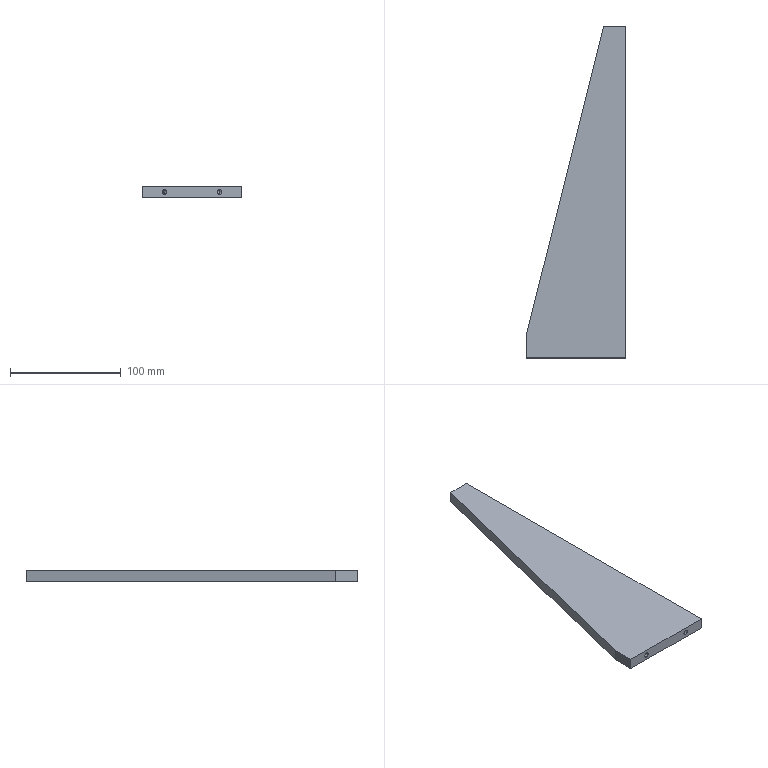Part | SolidWorks | features HoleWzd 2, Extrusion 1, ICE 1 | 1 solid | 23 faces | box 90 x 300 x 10 mm | volume 171179 mm3 | cylinder 8 | cone 8 | plane 7 | commonest cylinder face diameters 4.2 x8
STEP:
#1=CARTESIAN_POINT('',(30.6,110.,7.1));
#2=VERTEX_POINT('',#1);
#3=CARTESIAN_POINT('',(30.6,110.,2.9));
#4=VERTEX_POINT('',#3);
#5=CARTESIAN_POINT('',(30.6,110.,5.));
#6=DIRECTION('',(1.,0.,0.));
#7=DIRECTION('',(0.,0.,-1.));
#8=AXIS2_PLACEMENT_3D('',#5,#6,#7);
#9=CIRCLE('',#8,2.1);
#10=EDGE_CURVE('',#2,#4,#9,.T.);
#11=ORIENTED_EDGE('',*,*,#10,.F.);
#12=CARTESIAN_POINT('',(45.,110.,7.1));
#13=VERTEX_POINT('',#12);
#14=CARTESIAN_POINT('',(45.,110.,7.1));
#15=DIRECTION('',(1.,0.,0.));
#16=VECTOR('',#15,1000.);
#17=LINE('',#14,#16);
#18=EDGE_CURVE('',#2,#13,#17,.T.);
#19=ORIENTED_EDGE('',*,*,#18,.T.);
#20=CARTESIAN_POINT('',(45.,110.,2.9));
#21=VERTEX_POINT('',#20);
#22=CARTESIAN_POINT('',(45.,110.,5.));
#23=DIRECTION('',(1.,0.,0.));
#24=DIRECTION('',(0.,0.,-1.));
#25=AXIS2_PLACEMENT_3D('',#22,#23,#24);
#26=CIRCLE('',#25,2.1);
#27=EDGE_CURVE('',#13,#21,#26,.T.);
#28=ORIENTED_EDGE('',*,*,#27,.T.);
#29=CARTESIAN_POINT('',(45.,110.,2.9));
#30=DIRECTION('',(1.,0.,0.));
#31=VECTOR('',#30,1000.);
#32=LINE('',#29,#31);
#33=EDGE_CURVE('',#4,#21,#32,.T.);
#34=ORIENTED_EDGE('',*,*,#33,.F.);
#35=EDGE_LOOP('',(#11,#19,#28,#34));
#36=FACE_OUTER_BOUND('',#35,.T.);
#37=CARTESIAN_POINT('',(45.,110.,5.));
#38=DIRECTION('',(1.,0.,0.));
#39=DIRECTION('',(0.,0.,-1.));
#40=AXIS2_PLACEMENT_3D('',#37,#38,#39);
#41=CYLINDRICAL_SURFACE('',#40,2.1);
#42=ADVANCED_FACE('',(#36),#41,.F.);
#43=CARTESIAN_POINT('',(29.338,110.,5.));
#44=VERTEX_POINT('',#43);
#45=CARTESIAN_POINT('',(30.6,110.,2.9));
#46=DIRECTION('',(0.515,0.,-0.8572));
#47=VECTOR('',#46,1000.);
#48=LINE('',#45,#47);
#49=EDGE_CURVE('',#44,#4,#48,.T.);
#50=ORIENTED_EDGE('',*,*,#49,.F.);
#51=CARTESIAN_POINT('',(30.6,110.,7.1));
#52=DIRECTION('',(0.515,0.,0.8572));
#53=VECTOR('',#52,1000.);
#54=LINE('',#51,#53);
#55=EDGE_CURVE('',#44,#2,#54,.T.);
#56=ORIENTED_EDGE('',*,*,#55,.T.);
#57=ORIENTED_EDGE('',*,*,#10,.T.);
#58=EDGE_LOOP('',(#50,#56,#57));
#59=FACE_OUTER_BOUND('',#58,.T.);
#60=CARTESIAN_POINT('',(30.6,110.,5.));
#61=DIRECTION('',(1.,0.,0.));
#62=DIRECTION('',(0.,0.,-1.));
#63=AXIS2_PLACEMENT_3D('',#60,#61,#62);
#64=CONICAL_SURFACE('',#63,2.1,1.03);
#65=ADVANCED_FACE('',(#59),#64,.F.);
#66=CARTESIAN_POINT('',(30.6,10.,7.1));
#67=VERTEX_POINT('',#66);
#68=CARTESIAN_POINT('',(30.6,10.,2.9));
#69=VERTEX_POINT('',#68);
#70=CARTESIAN_POINT('',(30.6,10.,5.));
#71=DIRECTION('',(1.,0.,0.));
#72=DIRECTION('',(0.,0.,-1.));
#73=AXIS2_PLACEMENT_3D('',#70,#71,#72);
#74=CIRCLE('',#73,2.1);
#75=EDGE_CURVE('',#67,#69,#74,.T.);
#76=ORIENTED_EDGE('',*,*,#75,.F.);
#77=CARTESIAN_POINT('',(45.,10.,7.1));
#78=VERTEX_POINT('',#77);
#79=CARTESIAN_POINT('',(45.,10.,7.1));
#80=DIRECTION('',(1.,0.,0.));
#81=VECTOR('',#80,1000.);
#82=LINE('',#79,#81);
#83=EDGE_CURVE('',#67,#78,#82,.T.);
#84=ORIENTED_EDGE('',*,*,#83,.T.);
#85=CARTESIAN_POINT('',(45.,10.,2.9));
#86=VERTEX_POINT('',#85);
#87=CARTESIAN_POINT('',(45.,10.,5.));
#88=DIRECTION('',(1.,0.,0.));
#89=DIRECTION('',(0.,0.,-1.));
#90=AXIS2_PLACEMENT_3D('',#87,#88,#89);
#91=CIRCLE('',#90,2.1);
#92=EDGE_CURVE('',#78,#86,#91,.T.);
#93=ORIENTED_EDGE('',*,*,#92,.T.);
#94=CARTESIAN_POINT('',(45.,10.,2.9));
#95=DIRECTION('',(1.,0.,0.));
#96=VECTOR('',#95,1000.);
#97=LINE('',#94,#96);
#98=EDGE_CURVE('',#69,#86,#97,.T.);
#99=ORIENTED_EDGE('',*,*,#98,.F.);
#100=EDGE_LOOP('',(#76,#84,#93,#99));
#101=FACE_OUTER_BOUND('',#100,.T.);
#102=CARTESIAN_POINT('',(45.,10.,5.));
#103=DIRECTION('',(1.,0.,0.));
#104=DIRECTION('',(0.,0.,-1.));
#105=AXIS2_PLACEMENT_3D('',#102,#103,#104);
#106=CYLINDRICAL_SURFACE('',#105,2.1);
#107=ADVANCED_FACE('',(#101),#106,.F.);
#108=CARTESIAN_POINT('',(29.338,10.,5.));
#109=VERTEX_POINT('',#108);
#110=CARTESIAN_POINT('',(30.6,10.,2.9));
#111=DIRECTION('',(0.515,0.,-0.8572));
#112=VECTOR('',#111,1000.);
#113=LINE('',#110,#112);
#114=EDGE_CURVE('',#109,#69,#113,.T.);
#115=ORIENTED_EDGE('',*,*,#114,.F.);
#116=CARTESIAN_POINT('',(30.6,10.,7.1));
#117=DIRECTION('',(0.515,0.,0.8572));
#118=VECTOR('',#117,1000.);
#119=LINE('',#116,#118);
#120=EDGE_CURVE('',#109,#67,#119,.T.);
#121=ORIENTED_EDGE('',*,*,#120,.T.);
#122=ORIENTED_EDGE('',*,*,#75,.T.);
#123=EDGE_LOOP('',(#115,#121,#122));
#124=FACE_OUTER_BOUND('',#123,.T.);
#125=CARTESIAN_POINT('',(30.6,10.,5.));
#126=DIRECTION('',(1.,0.,0.));
#127=DIRECTION('',(0.,0.,-1.));
#128=AXIS2_PLACEMENT_3D('',#125,#126,#127);
#129=CONICAL_SURFACE('',#128,2.1,1.03);
#130=ADVANCED_FACE('',(#124),#129,.F.);
#131=CARTESIAN_POINT('',(25.,-135.6,7.1));
#132=VERTEX_POINT('',#131);
#133=CARTESIAN_POINT('',(25.,-135.6,2.9));
#134=VERTEX_POINT('',#133);
#135=CARTESIAN_POINT('',(25.,-135.6,5.));
#136=DIRECTION('',(0.,-1.,0.));
#137=DIRECTION('',(0.,0.,-1.));
#138=AXIS2_PLACEMENT_3D('',#135,#136,#137);
#139=CIRCLE('',#138,2.1);
#140=EDGE_CURVE('',#132,#134,#139,.T.);
#141=ORIENTED_EDGE('',*,*,#140,.F.);
#142=CARTESIAN_POINT('',(25.,-150.,7.1));
#143=VERTEX_POINT('',#142);
#144=CARTESIAN_POINT('',(25.,-150.,7.1));
#145=DIRECTION('',(0.,-1.,0.));
#146=VECTOR('',#145,1000.);
#147=LINE('',#144,#146);
#148=EDGE_CURVE('',#132,#143,#147,.T.);
#149=ORIENTED_EDGE('',*,*,#148,.T.);
#150=CARTESIAN_POINT('',(25.,-150.,2.9));
#151=VERTEX_POINT('',#150);
#152=CARTESIAN_POINT('',(25.,-150.,5.));
#153=DIRECTION('',(0.,-1.,0.));
#154=DIRECTION('',(0.,0.,-1.));
#155=AXIS2_PLACEMENT_3D('',#152,#153,#154);
#156=CIRCLE('',#155,2.1);
#157=EDGE_CURVE('',#143,#151,#156,.T.);
#158=ORIENTED_EDGE('',*,*,#157,.T.);
#159=CARTESIAN_POINT('',(25.,-150.,2.9));
#160=DIRECTION('',(0.,-1.,0.));
#161=VECTOR('',#160,1000.);
#162=LINE('',#159,#161);
#163=EDGE_CURVE('',#134,#151,#162,.T.);
#164=ORIENTED_EDGE('',*,*,#163,.F.);
#165=EDGE_LOOP('',(#141,#149,#158,#164));
#166=FACE_OUTER_BOUND('',#165,.T.);
#167=CARTESIAN_POINT('',(25.,-150.,5.));
#168=DIRECTION('',(0.,-1.,0.));
#169=DIRECTION('',(0.,0.,-1.));
#170=AXIS2_PLACEMENT_3D('',#167,#168,#169);
#171=CYLINDRICAL_SURFACE('',#170,2.1);
#172=ADVANCED_FACE('',(#166),#171,.F.);
#173=CARTESIAN_POINT('',(25.,-134.338,5.));
#174=VERTEX_POINT('',#173);
#175=CARTESIAN_POINT('',(25.,-135.6,2.9));
#176=DIRECTION('',(0.,-0.515,-0.8572));
#177=VECTOR('',#176,1000.);
#178=LINE('',#175,#177);
#179=EDGE_CURVE('',#174,#134,#178,.T.);
#180=ORIENTED_EDGE('',*,*,#179,.F.);
#181=CARTESIAN_POINT('',(25.,-135.6,7.1));
#182=DIRECTION('',(0.,-0.515,0.8572));
#183=VECTOR('',#182,1000.);
#184=LINE('',#181,#183);
#185=EDGE_CURVE('',#174,#132,#184,.T.);
#186=ORIENTED_EDGE('',*,*,#185,.T.);
#187=ORIENTED_EDGE('',*,*,#140,.T.);
#188=EDGE_LOOP('',(#180,#186,#187));
#189=FACE_OUTER_BOUND('',#188,.T.);
#190=CARTESIAN_POINT('',(25.,-135.6,5.));
#191=DIRECTION('',(0.,-1.,0.));
#192=DIRECTION('',(0.,0.,-1.));
#193=AXIS2_PLACEMENT_3D('',#190,#191,#192);
#194=CONICAL_SURFACE('',#193,2.1,1.03);
#195=ADVANCED_FACE('',(#189),#194,.F.);
#196=CARTESIAN_POINT('',(-25.,-135.6,7.1));
#197=VERTEX_POINT('',#196);
#198=CARTESIAN_POINT('',(-25.,-135.6,2.9));
#199=VERTEX_POINT('',#198);
#200=CARTESIAN_POINT('',(-25.,-135.6,5.));
#201=DIRECTION('',(0.,-1.,0.));
#202=DIRECTION('',(0.,0.,-1.));
#203=AXIS2_PLACEMENT_3D('',#200,#201,#202);
#204=CIRCLE('',#203,2.1);
#205=EDGE_CURVE('',#197,#199,#204,.T.);
#206=ORIENTED_EDGE('',*,*,#205,.F.);
#207=CARTESIAN_POINT('',(-25.,-150.,7.1));
#208=VERTEX_POINT('',#207);
#209=CARTESIAN_POINT('',(-25.,-150.,7.1));
#210=DIRECTION('',(0.,-1.,0.));
#211=VECTOR('',#210,1000.);
#212=LINE('',#209,#211);
#213=EDGE_CURVE('',#197,#208,#212,.T.);
#214=ORIENTED_EDGE('',*,*,#213,.T.);
#215=CARTESIAN_POINT('',(-25.,-150.,2.9));
#216=VERTEX_POINT('',#215);
#217=CARTESIAN_POINT('',(-25.,-150.,5.));
#218=DIRECTION('',(0.,-1.,0.));
#219=DIRECTION('',(0.,0.,-1.));
#220=AXIS2_PLACEMENT_3D('',#217,#218,#219);
#221=CIRCLE('',#220,2.1);
#222=EDGE_CURVE('',#208,#216,#221,.T.);
#223=ORIENTED_EDGE('',*,*,#222,.T.);
#224=CARTESIAN_POINT('',(-25.,-150.,2.9));
#225=DIRECTION('',(0.,-1.,0.));
#226=VECTOR('',#225,1000.);
#227=LINE('',#224,#226);
#228=EDGE_CURVE('',#199,#216,#227,.T.);
#229=ORIENTED_EDGE('',*,*,#228,.F.);
#230=EDGE_LOOP('',(#206,#214,#223,#229));
#231=FACE_OUTER_BOUND('',#230,.T.);
#232=CARTESIAN_POINT('',(-25.,-150.,5.));
#233=DIRECTION('',(0.,-1.,0.));
#234=DIRECTION('',(0.,0.,-1.));
#235=AXIS2_PLACEMENT_3D('',#232,#233,#234);
#236=CYLINDRICAL_SURFACE('',#235,2.1);
#237=ADVANCED_FACE('',(#231),#236,.F.);
#238=CARTESIAN_POINT('',(-25.,-134.338,5.));
#239=VERTEX_POINT('',#238);
#240=CARTESIAN_POINT('',(-25.,-135.6,2.9));
#241=DIRECTION('',(0.,-0.515,-0.8572));
#242=VECTOR('',#241,1000.);
#243=LINE('',#240,#242);
#244=EDGE_CURVE('',#239,#199,#243,.T.);
#245=ORIENTED_EDGE('',*,*,#244,.F.);
#246=CARTESIAN_POINT('',(-25.,-135.6,7.1));
#247=DIRECTION('',(0.,-0.515,0.8572));
#248=VECTOR('',#247,1000.);
#249=LINE('',#246,#248);
#250=EDGE_CURVE('',#239,#197,#249,.T.);
#251=ORIENTED_EDGE('',*,*,#250,.T.);
#252=ORIENTED_EDGE('',*,*,#205,.T.);
#253=EDGE_LOOP('',(#245,#251,#252));
#254=FACE_OUTER_BOUND('',#253,.T.);
#255=CARTESIAN_POINT('',(-25.,-135.6,5.));
#256=DIRECTION('',(0.,-1.,0.));
#257=DIRECTION('',(0.,0.,-1.));
#258=AXIS2_PLACEMENT_3D('',#255,#256,#257);
#259=CONICAL_SURFACE('',#258,2.1,1.03);
#260=ADVANCED_FACE('',(#254),#259,.F.);
#261=CARTESIAN_POINT('',(-45.,-130.,10.));
#262=VERTEX_POINT('',#261);
#263=CARTESIAN_POINT('',(-45.,-150.,10.));
#264=VERTEX_POINT('',#263);
#265=CARTESIAN_POINT('',(-45.,-150.,10.));
#266=DIRECTION('',(0.,-1.,0.));
#267=VECTOR('',#266,1000.);
#268=LINE('',#265,#267);
#269=EDGE_CURVE('',#262,#264,#268,.T.);
#270=ORIENTED_EDGE('',*,*,#269,.F.);
#271=CARTESIAN_POINT('',(-45.,-130.,0.));
#272=VERTEX_POINT('',#271);
#273=CARTESIAN_POINT('',(-45.,-130.,-0.001));
#274=DIRECTION('',(0.,0.,1.));
#275=VECTOR('',#274,1000.);
#276=LINE('',#273,#275);
#277=EDGE_CURVE('',#272,#262,#276,.T.);
#278=ORIENTED_EDGE('',*,*,#277,.F.);
#279=CARTESIAN_POINT('',(-45.,-150.,0.));
#280=VERTEX_POINT('',#279);
#281=CARTESIAN_POINT('',(-45.,-150.,0.));
#282=DIRECTION('',(0.,-1.,0.));
#283=VECTOR('',#282,1000.);
#284=LINE('',#281,#283);
#285=EDGE_CURVE('',#272,#280,#284,.T.);
#286=ORIENTED_EDGE('',*,*,#285,.T.);
#287=CARTESIAN_POINT('',(-45.,-150.,10.));
#288=DIRECTION('',(0.,0.,-1.));
#289=VECTOR('',#288,1000.);
#290=LINE('',#287,#289);
#291=EDGE_CURVE('',#264,#280,#290,.T.);
#292=ORIENTED_EDGE('',*,*,#291,.F.);
#293=EDGE_LOOP('',(#270,#278,#286,#292));
#294=FACE_OUTER_BOUND('',#293,.T.);
#295=CARTESIAN_POINT('',(-45.,-150.,10.));
#296=DIRECTION('',(1.,0.,0.));
#297=DIRECTION('',(0.,0.,-1.));
#298=AXIS2_PLACEMENT_3D('',#295,#296,#297);
#299=PLANE('',#298);
#300=ADVANCED_FACE('',(#294),#299,.F.);
#301=CARTESIAN_POINT('',(25.,-150.,5.));
#302=DIRECTION('',(0.,-1.,0.));
#303=DIRECTION('',(0.,0.,-1.));
#304=AXIS2_PLACEMENT_3D('',#301,#302,#303);
#305=CIRCLE('',#304,2.1);
#306=EDGE_CURVE('',#151,#143,#305,.T.);
#307=ORIENTED_EDGE('',*,*,#306,.F.);
#308=ORIENTED_EDGE('',*,*,#157,.F.);
#309=EDGE_LOOP('',(#307,#308));
#310=FACE_BOUND('',#309,.T.);
#311=CARTESIAN_POINT('',(-25.,-150.,5.));
#312=DIRECTION('',(0.,-1.,0.));
#313=DIRECTION('',(0.,0.,-1.));
#314=AXIS2_PLACEMENT_3D('',#311,#312,#313);
#315=CIRCLE('',#314,2.1);
#316=EDGE_CURVE('',#216,#208,#315,.T.);
#317=ORIENTED_EDGE('',*,*,#316,.F.);
#318=ORIENTED_EDGE('',*,*,#222,.F.);
#319=EDGE_LOOP('',(#317,#318));
#320=FACE_BOUND('',#319,.T.);
#321=CARTESIAN_POINT('',(45.,-150.,0.));
#322=VERTEX_POINT('',#321);
#323=CARTESIAN_POINT('',(45.,-150.,0.));
#324=DIRECTION('',(1.,0.,0.));
#325=VECTOR('',#324,1000.);
#326=LINE('',#323,#325);
#327=EDGE_CURVE('',#280,#322,#326,.T.);
#328=ORIENTED_EDGE('',*,*,#327,.T.);
#329=CARTESIAN_POINT('',(45.,-150.,10.));
#330=VERTEX_POINT('',#329);
#331=CARTESIAN_POINT('',(45.,-150.,10.));
#332=DIRECTION('',(0.,0.,-1.));
#333=VECTOR('',#332,1000.);
#334=LINE('',#331,#333);
#335=EDGE_CURVE('',#330,#322,#334,.T.);
#336=ORIENTED_EDGE('',*,*,#335,.F.);
#337=CARTESIAN_POINT('',(45.,-150.,10.));
#338=DIRECTION('',(1.,0.,0.));
#339=VECTOR('',#338,1000.);
#340=LINE('',#337,#339);
#341=EDGE_CURVE('',#264,#330,#340,.T.);
#342=ORIENTED_EDGE('',*,*,#341,.F.);
#343=ORIENTED_EDGE('',*,*,#291,.T.);
#344=EDGE_LOOP('',(#328,#336,#342,#343));
#345=FACE_OUTER_BOUND('',#344,.T.);
#346=CARTESIAN_POINT('',(45.,-150.,10.));
#347=DIRECTION('',(0.,1.,0.));
#348=DIRECTION('',(0.,0.,1.));
#349=AXIS2_PLACEMENT_3D('',#346,#347,#348);
#350=PLANE('',#349);
#351=ADVANCED_FACE('',(#310,#320,#345),#350,.F.);
#352=CARTESIAN_POINT('',(45.,110.,5.));
#353=DIRECTION('',(1.,0.,0.));
#354=DIRECTION('',(0.,0.,-1.));
#355=AXIS2_PLACEMENT_3D('',#352,#353,#354);
#356=CIRCLE('',#355,2.1);
#357=EDGE_CURVE('',#21,#13,#356,.T.);
#358=ORIENTED_EDGE('',*,*,#357,.F.);
#359=ORIENTED_EDGE('',*,*,#27,.F.);
#360=EDGE_LOOP('',(#358,#359));
#361=FACE_BOUND('',#360,.T.);
#362=CARTESIAN_POINT('',(45.,10.,5.));
#363=DIRECTION('',(1.,0.,0.));
#364=DIRECTION('',(0.,0.,-1.));
#365=AXIS2_PLACEMENT_3D('',#362,#363,#364);
#366=CIRCLE('',#365,2.1);
#367=EDGE_CURVE('',#86,#78,#366,.T.);
#368=ORIENTED_EDGE('',*,*,#367,.F.);
#369=ORIENTED_EDGE('',*,*,#92,.F.);
#370=EDGE_LOOP('',(#368,#369));
#371=FACE_BOUND('',#370,.T.);
#372=CARTESIAN_POINT('',(45.,150.,0.));
#373=VERTEX_POINT('',#372);
#374=CARTESIAN_POINT('',(45.,-150.,0.));
#375=DIRECTION('',(0.,1.,0.));
#376=VECTOR('',#375,1000.);
#377=LINE('',#374,#376);
#378=EDGE_CURVE('',#322,#373,#377,.T.);
#379=ORIENTED_EDGE('',*,*,#378,.T.);
#380=CARTESIAN_POINT('',(45.,150.,10.));
#381=VERTEX_POINT('',#380);
#382=CARTESIAN_POINT('',(45.,150.,10.));
#383=DIRECTION('',(0.,0.,-1.));
#384=VECTOR('',#383,1000.);
#385=LINE('',#382,#384);
#386=EDGE_CURVE('',#381,#373,#385,.T.);
#387=ORIENTED_EDGE('',*,*,#386,.F.);
#388=CARTESIAN_POINT('',(45.,-150.,10.));
#389=DIRECTION('',(0.,1.,0.));
#390=VECTOR('',#389,1000.);
#391=LINE('',#388,#390);
#392=EDGE_CURVE('',#330,#381,#391,.T.);
#393=ORIENTED_EDGE('',*,*,#392,.F.);
#394=ORIENTED_EDGE('',*,*,#335,.T.);
#395=EDGE_LOOP('',(#379,#387,#393,#394));
#396=FACE_OUTER_BOUND('',#395,.T.);
#397=CARTESIAN_POINT('',(45.,-150.,10.));
#398=DIRECTION('',(-1.,0.,0.));
#399=DIRECTION('',(0.,0.,1.));
#400=AXIS2_PLACEMENT_3D('',#397,#398,#399);
#401=PLANE('',#400);
#402=ADVANCED_FACE('',(#361,#371,#396),#401,.F.);
#403=CARTESIAN_POINT('',(25.,150.,0.));
#404=VERTEX_POINT('',#403);
#405=CARTESIAN_POINT('',(45.,150.,0.));
#406=DIRECTION('',(-1.,0.,0.));
#407=VECTOR('',#406,1000.);
#408=LINE('',#405,#407);
#409=EDGE_CURVE('',#373,#404,#408,.T.);
#410=ORIENTED_EDGE('',*,*,#409,.T.);
#411=CARTESIAN_POINT('',(25.,150.,10.));
#412=VERTEX_POINT('',#411);
#413=CARTESIAN_POINT('',(25.,150.,-0.001));
#414=DIRECTION('',(0.,0.,1.));
#415=VECTOR('',#414,1000.);
#416=LINE('',#413,#415);
#417=EDGE_CURVE('',#404,#412,#416,.T.);
#418=ORIENTED_EDGE('',*,*,#417,.T.);
#419=CARTESIAN_POINT('',(45.,150.,10.));
#420=DIRECTION('',(-1.,0.,0.));
#421=VECTOR('',#420,1000.);
#422=LINE('',#419,#421);
#423=EDGE_CURVE('',#381,#412,#422,.T.);
#424=ORIENTED_EDGE('',*,*,#423,.F.);
#425=ORIENTED_EDGE('',*,*,#386,.T.);
#426=EDGE_LOOP('',(#410,#418,#424,#425));
#427=FACE_OUTER_BOUND('',#426,.T.);
#428=CARTESIAN_POINT('',(45.,150.,10.));
#429=DIRECTION('',(0.,-1.,0.));
#430=DIRECTION('',(0.,0.,-1.));
#431=AXIS2_PLACEMENT_3D('',#428,#429,#430);
#432=PLANE('',#431);
#433=ADVANCED_FACE('',(#427),#432,.F.);
#434=CARTESIAN_POINT('',(-45.,-130.,10.));
#435=DIRECTION('',(0.2425,0.9701,0.));
#436=VECTOR('',#435,1000.);
#437=LINE('',#434,#436);
#438=EDGE_CURVE('',#262,#412,#437,.T.);
#439=ORIENTED_EDGE('',*,*,#438,.F.);
#440=ORIENTED_EDGE('',*,*,#269,.T.);
#441=ORIENTED_EDGE('',*,*,#341,.T.);
#442=ORIENTED_EDGE('',*,*,#392,.T.);
#443=ORIENTED_EDGE('',*,*,#423,.T.);
#444=EDGE_LOOP('',(#439,#440,#441,#442,#443));
#445=FACE_OUTER_BOUND('',#444,.T.);
#446=CARTESIAN_POINT('',(0.,0.,10.));
#447=DIRECTION('',(0.,0.,1.));
#448=DIRECTION('',(1.,0.,0.));
#449=AXIS2_PLACEMENT_3D('',#446,#447,#448);
#450=PLANE('',#449);
#451=ADVANCED_FACE('',(#445),#450,.T.);
#452=ORIENTED_EDGE('',*,*,#285,.F.);
#453=CARTESIAN_POINT('',(-45.,-130.,0.));
#454=DIRECTION('',(-0.2425,-0.9701,0.));
#455=VECTOR('',#454,1000.);
#456=LINE('',#453,#455);
#457=EDGE_CURVE('',#404,#272,#456,.T.);
#458=ORIENTED_EDGE('',*,*,#457,.F.);
#459=ORIENTED_EDGE('',*,*,#409,.F.);
#460=ORIENTED_EDGE('',*,*,#378,.F.);
#461=ORIENTED_EDGE('',*,*,#327,.F.);
#462=EDGE_LOOP('',(#452,#458,#459,#460,#461));
#463=FACE_OUTER_BOUND('',#462,.T.);
#464=CARTESIAN_POINT('',(0.,0.,0.));
#465=DIRECTION('',(0.,0.,1.));
#466=DIRECTION('',(1.,0.,0.));
#467=AXIS2_PLACEMENT_3D('',#464,#465,#466);
#468=PLANE('',#467);
#469=ADVANCED_FACE('',(#463),#468,.F.);
#470=ORIENTED_EDGE('',*,*,#457,.T.);
#471=ORIENTED_EDGE('',*,*,#277,.T.);
#472=ORIENTED_EDGE('',*,*,#438,.T.);
#473=ORIENTED_EDGE('',*,*,#417,.F.);
#474=EDGE_LOOP('',(#470,#471,#472,#473));
#475=FACE_OUTER_BOUND('',#474,.T.);
#476=CARTESIAN_POINT('',(-45.,-130.,-0.001));
#477=DIRECTION('',(0.9701,-0.2425,0.));
#478=DIRECTION('',(0.2425,0.9701,0.));
#479=AXIS2_PLACEMENT_3D('',#476,#477,#478);
#480=PLANE('',#479);
#481=ADVANCED_FACE('',(#475),#480,.F.);
#482=ORIENTED_EDGE('',*,*,#250,.F.);
#483=ORIENTED_EDGE('',*,*,#244,.T.);
#484=CARTESIAN_POINT('',(-25.,-135.6,5.));
#485=DIRECTION('',(0.,-1.,0.));
#486=DIRECTION('',(0.,0.,-1.));
#487=AXIS2_PLACEMENT_3D('',#484,#485,#486);
#488=CIRCLE('',#487,2.1);
#489=EDGE_CURVE('',#199,#197,#488,.T.);
#490=ORIENTED_EDGE('',*,*,#489,.T.);
#491=EDGE_LOOP('',(#482,#483,#490));
#492=FACE_OUTER_BOUND('',#491,.T.);
#493=CARTESIAN_POINT('',(-25.,-135.6,5.));
#494=DIRECTION('',(0.,-1.,0.));
#495=DIRECTION('',(0.,0.,-1.));
#496=AXIS2_PLACEMENT_3D('',#493,#494,#495);
#497=CONICAL_SURFACE('',#496,2.1,1.03);
#498=ADVANCED_FACE('',(#492),#497,.F.);
#499=ORIENTED_EDGE('',*,*,#213,.F.);
#500=ORIENTED_EDGE('',*,*,#489,.F.);
#501=ORIENTED_EDGE('',*,*,#228,.T.);
#502=ORIENTED_EDGE('',*,*,#316,.T.);
#503=EDGE_LOOP('',(#499,#500,#501,#502));
#504=FACE_OUTER_BOUND('',#503,.T.);
#505=CARTESIAN_POINT('',(-25.,-150.,5.));
#506=DIRECTION('',(0.,-1.,0.));
#507=DIRECTION('',(0.,0.,-1.));
#508=AXIS2_PLACEMENT_3D('',#505,#506,#507);
#509=CYLINDRICAL_SURFACE('',#508,2.1);
#510=ADVANCED_FACE('',(#504),#509,.F.);
#511=ORIENTED_EDGE('',*,*,#185,.F.);
#512=ORIENTED_EDGE('',*,*,#179,.T.);
#513=CARTESIAN_POINT('',(25.,-135.6,5.));
#514=DIRECTION('',(0.,-1.,0.));
#515=DIRECTION('',(0.,0.,-1.));
#516=AXIS2_PLACEMENT_3D('',#513,#514,#515);
#517=CIRCLE('',#516,2.1);
#518=EDGE_CURVE('',#134,#132,#517,.T.);
#519=ORIENTED_EDGE('',*,*,#518,.T.);
#520=EDGE_LOOP('',(#511,#512,#519));
#521=FACE_OUTER_BOUND('',#520,.T.);
#522=CARTESIAN_POINT('',(25.,-135.6,5.));
#523=DIRECTION('',(0.,-1.,0.));
#524=DIRECTION('',(0.,0.,-1.));
#525=AXIS2_PLACEMENT_3D('',#522,#523,#524);
#526=CONICAL_SURFACE('',#525,2.1,1.03);
#527=ADVANCED_FACE('',(#521),#526,.F.);
#528=ORIENTED_EDGE('',*,*,#148,.F.);
#529=ORIENTED_EDGE('',*,*,#518,.F.);
#530=ORIENTED_EDGE('',*,*,#163,.T.);
#531=ORIENTED_EDGE('',*,*,#306,.T.);
#532=EDGE_LOOP('',(#528,#529,#530,#531));
#533=FACE_OUTER_BOUND('',#532,.T.);
#534=CARTESIAN_POINT('',(25.,-150.,5.));
#535=DIRECTION('',(0.,-1.,0.));
#536=DIRECTION('',(0.,0.,-1.));
#537=AXIS2_PLACEMENT_3D('',#534,#535,#536);
#538=CYLINDRICAL_SURFACE('',#537,2.1);
#539=ADVANCED_FACE('',(#533),#538,.F.);
#540=ORIENTED_EDGE('',*,*,#120,.F.);
#541=ORIENTED_EDGE('',*,*,#114,.T.);
#542=CARTESIAN_POINT('',(30.6,10.,5.));
#543=DIRECTION('',(1.,0.,0.));
#544=DIRECTION('',(0.,0.,-1.));
#545=AXIS2_PLACEMENT_3D('',#542,#543,#544);
#546=CIRCLE('',#545,2.1);
#547=EDGE_CURVE('',#69,#67,#546,.T.);
#548=ORIENTED_EDGE('',*,*,#547,.T.);
#549=EDGE_LOOP('',(#540,#541,#548));
#550=FACE_OUTER_BOUND('',#549,.T.);
#551=CARTESIAN_POINT('',(30.6,10.,5.));
#552=DIRECTION('',(1.,0.,0.));
#553=DIRECTION('',(0.,0.,-1.));
#554=AXIS2_PLACEMENT_3D('',#551,#552,#553);
#555=CONICAL_SURFACE('',#554,2.1,1.03);
#556=ADVANCED_FACE('',(#550),#555,.F.);
#557=ORIENTED_EDGE('',*,*,#83,.F.);
#558=ORIENTED_EDGE('',*,*,#547,.F.);
#559=ORIENTED_EDGE('',*,*,#98,.T.);
#560=ORIENTED_EDGE('',*,*,#367,.T.);
#561=EDGE_LOOP('',(#557,#558,#559,#560));
#562=FACE_OUTER_BOUND('',#561,.T.);
#563=CARTESIAN_POINT('',(45.,10.,5.));
#564=DIRECTION('',(1.,0.,0.));
#565=DIRECTION('',(0.,0.,-1.));
#566=AXIS2_PLACEMENT_3D('',#563,#564,#565);
#567=CYLINDRICAL_SURFACE('',#566,2.1);
#568=ADVANCED_FACE('',(#562),#567,.F.);
#569=ORIENTED_EDGE('',*,*,#55,.F.);
#570=ORIENTED_EDGE('',*,*,#49,.T.);
#571=CARTESIAN_POINT('',(30.6,110.,5.));
#572=DIRECTION('',(1.,0.,0.));
#573=DIRECTION('',(0.,0.,-1.));
#574=AXIS2_PLACEMENT_3D('',#571,#572,#573);
#575=CIRCLE('',#574,2.1);
#576=EDGE_CURVE('',#4,#2,#575,.T.);
#577=ORIENTED_EDGE('',*,*,#576,.T.);
#578=EDGE_LOOP('',(#569,#570,#577));
#579=FACE_OUTER_BOUND('',#578,.T.);
#580=CARTESIAN_POINT('',(30.6,110.,5.));
#581=DIRECTION('',(1.,0.,0.));
#582=DIRECTION('',(0.,0.,-1.));
#583=AXIS2_PLACEMENT_3D('',#580,#581,#582);
#584=CONICAL_SURFACE('',#583,2.1,1.03);
#585=ADVANCED_FACE('',(#579),#584,.F.);
#586=ORIENTED_EDGE('',*,*,#18,.F.);
#587=ORIENTED_EDGE('',*,*,#576,.F.);
#588=ORIENTED_EDGE('',*,*,#33,.T.);
#589=ORIENTED_EDGE('',*,*,#357,.T.);
#590=EDGE_LOOP('',(#586,#587,#588,#589));
#591=FACE_OUTER_BOUND('',#590,.T.);
#592=CARTESIAN_POINT('',(45.,110.,5.));
#593=DIRECTION('',(1.,0.,0.));
#594=DIRECTION('',(0.,0.,-1.));
#595=AXIS2_PLACEMENT_3D('',#592,#593,#594);
#596=CYLINDRICAL_SURFACE('',#595,2.1);
#597=ADVANCED_FACE('',(#591),#596,.F.);
#598=CLOSED_SHELL('',(#42,#65,#107,#130,#172,#195,#237,#260,#300,#351,#402,#433,#451,#469,#481,#498,#510,#527,#539,#556,#568,#585,#597));
#599=MANIFOLD_SOLID_BREP('',#598);
#600=CARTESIAN_POINT('',(0.,0.,0.));
#601=DIRECTION('',(0.,0.,1.));
#602=DIRECTION('',(1.,0.,0.));
#603=AXIS2_PLACEMENT_3D('',#600,#601,#602);
#604=(LENGTH_UNIT()NAMED_UNIT(*)SI_UNIT(.MILLI.,.METRE.));
#605=UNCERTAINTY_MEASURE_WITH_UNIT(LENGTH_MEASURE(0.00001),#604,'','');
#606=(NAMED_UNIT(*)PLANE_ANGLE_UNIT()SI_UNIT($,.RADIAN.));
#607=(NAMED_UNIT(*)SI_UNIT($,.STERADIAN.)SOLID_ANGLE_UNIT());
#608=(GEOMETRIC_REPRESENTATION_CONTEXT(3)GLOBAL_UNCERTAINTY_ASSIGNED_CONTEXT((#605))GLOBAL_UNIT_ASSIGNED_CONTEXT((#604,#606,#607))REPRESENTATION_CONTEXT('',''));
#609=ADVANCED_BREP_SHAPE_REPRESENTATION('',(#599,#603),#608);